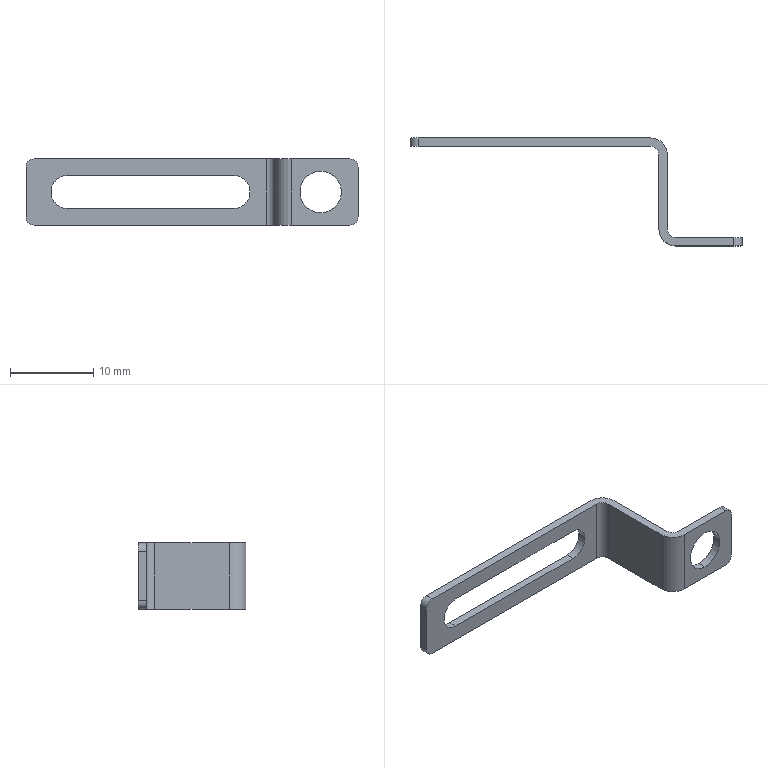Part | NX | features BREP 1 | 1 solid | 24 faces | box 40 x 13 x 8 mm | volume 292.639 mm3 | cylinder 12 | plane 12 | commonest cylinder face diameters 2 x6 4 x4 5 x2
STEP:
#1=CARTESIAN_POINT('',(5.5,0.,1.5));
#2=VERTEX_POINT('',#1);
#3=CARTESIAN_POINT('',(5.5,0.,6.5));
#4=VERTEX_POINT('',#3);
#5=CARTESIAN_POINT('',(5.5,0.,4.));
#6=DIRECTION('',(0.,1.,0.));
#7=DIRECTION('',(0.,0.,1.));
#8=AXIS2_PLACEMENT_3D('',#5,#6,#7);
#9=CIRCLE('',#8,2.5);
#10=EDGE_CURVE('',#2,#4,#9,.T.);
#11=ORIENTED_EDGE('',*,*,#10,.F.);
#12=CARTESIAN_POINT('',(5.5,1.,1.5));
#13=VERTEX_POINT('',#12);
#14=CARTESIAN_POINT('',(5.5,0.,1.5));
#15=DIRECTION('',(0.,1.,0.));
#16=VECTOR('',#15,1000.);
#17=LINE('',#14,#16);
#18=EDGE_CURVE('',#13,#2,#17,.F.);
#19=ORIENTED_EDGE('',*,*,#18,.F.);
#20=CARTESIAN_POINT('',(5.5,1.,6.5));
#21=VERTEX_POINT('',#20);
#22=CARTESIAN_POINT('',(5.5,1.,4.));
#23=DIRECTION('',(0.,1.,0.));
#24=DIRECTION('',(0.,0.,1.));
#25=AXIS2_PLACEMENT_3D('',#22,#23,#24);
#26=CIRCLE('',#25,2.5);
#27=EDGE_CURVE('',#13,#21,#26,.T.);
#28=ORIENTED_EDGE('',*,*,#27,.T.);
#29=CARTESIAN_POINT('',(5.5,0.,6.5));
#30=DIRECTION('',(0.,1.,0.));
#31=VECTOR('',#30,1000.);
#32=LINE('',#29,#31);
#33=EDGE_CURVE('',#21,#4,#32,.F.);
#34=ORIENTED_EDGE('',*,*,#33,.T.);
#35=EDGE_LOOP('',(#11,#19,#28,#34));
#36=FACE_BOUND('',#35,.T.);
#37=CARTESIAN_POINT('',(5.5,0.,4.));
#38=DIRECTION('',(0.,1.,0.));
#39=DIRECTION('',(0.,0.,1.));
#40=AXIS2_PLACEMENT_3D('',#37,#38,#39);
#41=CYLINDRICAL_SURFACE('',#40,2.5);
#42=ADVANCED_FACE('',(#36),#41,.F.);
#43=CARTESIAN_POINT('',(-1.,13.,8.));
#44=VERTEX_POINT('',#43);
#45=CARTESIAN_POINT('',(-29.,13.,8.));
#46=VERTEX_POINT('',#45);
#47=CARTESIAN_POINT('',(0.,13.,8.));
#48=DIRECTION('',(-1.,0.,0.));
#49=VECTOR('',#48,1000.);
#50=LINE('',#47,#49);
#51=EDGE_CURVE('',#44,#46,#50,.T.);
#52=ORIENTED_EDGE('',*,*,#51,.F.);
#53=CARTESIAN_POINT('',(-1.,13.,0.));
#54=VERTEX_POINT('',#53);
#55=CARTESIAN_POINT('',(-1.,13.,8.));
#56=DIRECTION('',(0.,0.,-1.));
#57=VECTOR('',#56,1000.);
#58=LINE('',#55,#57);
#59=EDGE_CURVE('',#44,#54,#58,.T.);
#60=ORIENTED_EDGE('',*,*,#59,.T.);
#61=CARTESIAN_POINT('',(-29.,13.,0.));
#62=VERTEX_POINT('',#61);
#63=CARTESIAN_POINT('',(0.,13.,0.));
#64=DIRECTION('',(-1.,0.,0.));
#65=VECTOR('',#64,1000.);
#66=LINE('',#63,#65);
#67=EDGE_CURVE('',#54,#62,#66,.T.);
#68=ORIENTED_EDGE('',*,*,#67,.T.);
#69=CARTESIAN_POINT('',(-30.,13.,1.));
#70=VERTEX_POINT('',#69);
#71=CARTESIAN_POINT('',(-29.,13.,1.));
#72=DIRECTION('',(0.,1.,0.));
#73=DIRECTION('',(1.,0.,0.));
#74=AXIS2_PLACEMENT_3D('',#71,#72,#73);
#75=CIRCLE('',#74,1.);
#76=EDGE_CURVE('',#62,#70,#75,.T.);
#77=ORIENTED_EDGE('',*,*,#76,.T.);
#78=CARTESIAN_POINT('',(-30.,13.,7.));
#79=VERTEX_POINT('',#78);
#80=CARTESIAN_POINT('',(-30.,13.,8.));
#81=DIRECTION('',(0.,0.,-1.));
#82=VECTOR('',#81,1000.);
#83=LINE('',#80,#82);
#84=EDGE_CURVE('',#79,#70,#83,.T.);
#85=ORIENTED_EDGE('',*,*,#84,.F.);
#86=CARTESIAN_POINT('',(-29.,13.,7.));
#87=DIRECTION('',(0.,1.,0.));
#88=DIRECTION('',(1.,0.,0.));
#89=AXIS2_PLACEMENT_3D('',#86,#87,#88);
#90=CIRCLE('',#89,1.);
#91=EDGE_CURVE('',#79,#46,#90,.T.);
#92=ORIENTED_EDGE('',*,*,#91,.T.);
#93=EDGE_LOOP('',(#52,#60,#68,#77,#85,#92));
#94=FACE_BOUND('',#93,.T.);
#95=CARTESIAN_POINT('',(-25.,13.,6.));
#96=VERTEX_POINT('',#95);
#97=CARTESIAN_POINT('',(-5.,13.,6.));
#98=VERTEX_POINT('',#97);
#99=CARTESIAN_POINT('',(-25.,13.,6.));
#100=DIRECTION('',(1.,0.,0.));
#101=VECTOR('',#100,1000.);
#102=LINE('',#99,#101);
#103=EDGE_CURVE('',#96,#98,#102,.T.);
#104=ORIENTED_EDGE('',*,*,#103,.F.);
#105=CARTESIAN_POINT('',(-25.,13.,2.));
#106=VERTEX_POINT('',#105);
#107=CARTESIAN_POINT('',(-25.,13.,4.));
#108=DIRECTION('',(0.,1.,0.));
#109=DIRECTION('',(0.,0.,1.));
#110=AXIS2_PLACEMENT_3D('',#107,#108,#109);
#111=CIRCLE('',#110,2.);
#112=EDGE_CURVE('',#106,#96,#111,.T.);
#113=ORIENTED_EDGE('',*,*,#112,.F.);
#114=CARTESIAN_POINT('',(-5.,13.,2.));
#115=VERTEX_POINT('',#114);
#116=CARTESIAN_POINT('',(-25.,13.,2.));
#117=DIRECTION('',(-1.,0.,0.));
#118=VECTOR('',#117,1000.);
#119=LINE('',#116,#118);
#120=EDGE_CURVE('',#115,#106,#119,.T.);
#121=ORIENTED_EDGE('',*,*,#120,.F.);
#122=CARTESIAN_POINT('',(-5.,13.,4.));
#123=DIRECTION('',(0.,1.,0.));
#124=DIRECTION('',(0.,0.,1.));
#125=AXIS2_PLACEMENT_3D('',#122,#123,#124);
#126=CIRCLE('',#125,2.);
#127=EDGE_CURVE('',#98,#115,#126,.T.);
#128=ORIENTED_EDGE('',*,*,#127,.F.);
#129=EDGE_LOOP('',(#104,#113,#121,#128));
#130=FACE_BOUND('',#129,.T.);
#131=CARTESIAN_POINT('',(0.,13.,8.));
#132=DIRECTION('',(0.,-1.,0.));
#133=DIRECTION('',(0.,0.,-1.));
#134=AXIS2_PLACEMENT_3D('',#131,#132,#133);
#135=PLANE('',#134);
#136=ADVANCED_FACE('',(#94,#130),#135,.F.);
#137=ORIENTED_EDGE('',*,*,#84,.T.);
#138=CARTESIAN_POINT('',(-30.,12.,1.));
#139=VERTEX_POINT('',#138);
#140=CARTESIAN_POINT('',(-30.,12.,1.));
#141=DIRECTION('',(0.,-1.,0.));
#142=VECTOR('',#141,1000.);
#143=LINE('',#140,#142);
#144=EDGE_CURVE('',#70,#139,#143,.T.);
#145=ORIENTED_EDGE('',*,*,#144,.T.);
#146=CARTESIAN_POINT('',(-30.,12.,7.));
#147=VERTEX_POINT('',#146);
#148=CARTESIAN_POINT('',(-30.,12.,8.));
#149=DIRECTION('',(0.,0.,-1.));
#150=VECTOR('',#149,1000.);
#151=LINE('',#148,#150);
#152=EDGE_CURVE('',#147,#139,#151,.T.);
#153=ORIENTED_EDGE('',*,*,#152,.F.);
#154=CARTESIAN_POINT('',(-30.,13.,7.));
#155=DIRECTION('',(0.,1.,0.));
#156=VECTOR('',#155,1000.);
#157=LINE('',#154,#156);
#158=EDGE_CURVE('',#147,#79,#157,.T.);
#159=ORIENTED_EDGE('',*,*,#158,.T.);
#160=EDGE_LOOP('',(#137,#145,#153,#159));
#161=FACE_BOUND('',#160,.T.);
#162=CARTESIAN_POINT('',(-30.,12.,8.));
#163=DIRECTION('',(-1.,0.,0.));
#164=DIRECTION('',(0.,0.,1.));
#165=AXIS2_PLACEMENT_3D('',#162,#163,#164);
#166=PLANE('',#165);
#167=ADVANCED_FACE('',(#161),#166,.T.);
#168=CARTESIAN_POINT('',(-1.,12.,0.));
#169=VERTEX_POINT('',#168);
#170=CARTESIAN_POINT('',(-29.,12.,0.));
#171=VERTEX_POINT('',#170);
#172=CARTESIAN_POINT('',(0.,12.,0.));
#173=DIRECTION('',(-1.,0.,0.));
#174=VECTOR('',#173,1000.);
#175=LINE('',#172,#174);
#176=EDGE_CURVE('',#169,#171,#175,.T.);
#177=ORIENTED_EDGE('',*,*,#176,.F.);
#178=CARTESIAN_POINT('',(-1.,12.,8.));
#179=VERTEX_POINT('',#178);
#180=CARTESIAN_POINT('',(-1.,12.,8.));
#181=DIRECTION('',(0.,0.,1.));
#182=VECTOR('',#181,1000.);
#183=LINE('',#180,#182);
#184=EDGE_CURVE('',#169,#179,#183,.T.);
#185=ORIENTED_EDGE('',*,*,#184,.T.);
#186=CARTESIAN_POINT('',(-29.,12.,8.));
#187=VERTEX_POINT('',#186);
#188=CARTESIAN_POINT('',(0.,12.,8.));
#189=DIRECTION('',(-1.,0.,0.));
#190=VECTOR('',#189,1000.);
#191=LINE('',#188,#190);
#192=EDGE_CURVE('',#179,#187,#191,.T.);
#193=ORIENTED_EDGE('',*,*,#192,.T.);
#194=CARTESIAN_POINT('',(-29.,12.,7.));
#195=DIRECTION('',(0.,-1.,0.));
#196=DIRECTION('',(1.,0.,0.));
#197=AXIS2_PLACEMENT_3D('',#194,#195,#196);
#198=CIRCLE('',#197,1.);
#199=EDGE_CURVE('',#187,#147,#198,.T.);
#200=ORIENTED_EDGE('',*,*,#199,.T.);
#201=ORIENTED_EDGE('',*,*,#152,.T.);
#202=CARTESIAN_POINT('',(-29.,12.,1.));
#203=DIRECTION('',(0.,-1.,0.));
#204=DIRECTION('',(1.,0.,0.));
#205=AXIS2_PLACEMENT_3D('',#202,#203,#204);
#206=CIRCLE('',#205,1.);
#207=EDGE_CURVE('',#139,#171,#206,.T.);
#208=ORIENTED_EDGE('',*,*,#207,.T.);
#209=EDGE_LOOP('',(#177,#185,#193,#200,#201,#208));
#210=FACE_BOUND('',#209,.T.);
#211=CARTESIAN_POINT('',(-25.,12.,6.));
#212=VERTEX_POINT('',#211);
#213=CARTESIAN_POINT('',(-25.,12.,2.));
#214=VERTEX_POINT('',#213);
#215=CARTESIAN_POINT('',(-25.,12.,4.));
#216=DIRECTION('',(0.,-1.,0.));
#217=DIRECTION('',(1.,0.,0.));
#218=AXIS2_PLACEMENT_3D('',#215,#216,#217);
#219=CIRCLE('',#218,2.);
#220=EDGE_CURVE('',#212,#214,#219,.T.);
#221=ORIENTED_EDGE('',*,*,#220,.F.);
#222=CARTESIAN_POINT('',(-5.,12.,6.));
#223=VERTEX_POINT('',#222);
#224=CARTESIAN_POINT('',(0.,12.,6.));
#225=DIRECTION('',(-1.,0.,0.));
#226=VECTOR('',#225,1000.);
#227=LINE('',#224,#226);
#228=EDGE_CURVE('',#223,#212,#227,.T.);
#229=ORIENTED_EDGE('',*,*,#228,.F.);
#230=CARTESIAN_POINT('',(-5.,12.,2.));
#231=VERTEX_POINT('',#230);
#232=CARTESIAN_POINT('',(-5.,12.,4.));
#233=DIRECTION('',(0.,-1.,0.));
#234=DIRECTION('',(1.,0.,0.));
#235=AXIS2_PLACEMENT_3D('',#232,#233,#234);
#236=CIRCLE('',#235,2.);
#237=EDGE_CURVE('',#231,#223,#236,.T.);
#238=ORIENTED_EDGE('',*,*,#237,.F.);
#239=CARTESIAN_POINT('',(0.,12.,2.));
#240=DIRECTION('',(1.,0.,0.));
#241=VECTOR('',#240,1000.);
#242=LINE('',#239,#241);
#243=EDGE_CURVE('',#214,#231,#242,.T.);
#244=ORIENTED_EDGE('',*,*,#243,.F.);
#245=EDGE_LOOP('',(#221,#229,#238,#244));
#246=FACE_BOUND('',#245,.T.);
#247=CARTESIAN_POINT('',(0.,12.,8.));
#248=DIRECTION('',(0.,-1.,0.));
#249=DIRECTION('',(0.,0.,-1.));
#250=AXIS2_PLACEMENT_3D('',#247,#248,#249);
#251=PLANE('',#250);
#252=ADVANCED_FACE('',(#210,#246),#251,.T.);
#253=CARTESIAN_POINT('',(0.,2.,0.));
#254=VERTEX_POINT('',#253);
#255=CARTESIAN_POINT('',(0.,11.,0.));
#256=VERTEX_POINT('',#255);
#257=CARTESIAN_POINT('',(0.,0.,0.));
#258=DIRECTION('',(0.,1.,0.));
#259=VECTOR('',#258,1000.);
#260=LINE('',#257,#259);
#261=EDGE_CURVE('',#254,#256,#260,.T.);
#262=ORIENTED_EDGE('',*,*,#261,.F.);
#263=CARTESIAN_POINT('',(0.,2.,8.));
#264=VERTEX_POINT('',#263);
#265=CARTESIAN_POINT('',(0.,2.,8.));
#266=DIRECTION('',(0.,0.,1.));
#267=VECTOR('',#266,1000.);
#268=LINE('',#265,#267);
#269=EDGE_CURVE('',#254,#264,#268,.T.);
#270=ORIENTED_EDGE('',*,*,#269,.T.);
#271=CARTESIAN_POINT('',(0.,11.,8.));
#272=VERTEX_POINT('',#271);
#273=CARTESIAN_POINT('',(0.,0.,8.));
#274=DIRECTION('',(0.,1.,0.));
#275=VECTOR('',#274,1000.);
#276=LINE('',#273,#275);
#277=EDGE_CURVE('',#264,#272,#276,.T.);
#278=ORIENTED_EDGE('',*,*,#277,.T.);
#279=CARTESIAN_POINT('',(0.,11.,0.));
#280=DIRECTION('',(0.,0.,-1.));
#281=VECTOR('',#280,1000.);
#282=LINE('',#279,#281);
#283=EDGE_CURVE('',#272,#256,#282,.T.);
#284=ORIENTED_EDGE('',*,*,#283,.T.);
#285=EDGE_LOOP('',(#262,#270,#278,#284));
#286=FACE_BOUND('',#285,.T.);
#287=CARTESIAN_POINT('',(0.,0.,8.));
#288=DIRECTION('',(-1.,0.,0.));
#289=DIRECTION('',(0.,0.,1.));
#290=AXIS2_PLACEMENT_3D('',#287,#288,#289);
#291=PLANE('',#290);
#292=ADVANCED_FACE('',(#286),#291,.T.);
#293=CARTESIAN_POINT('',(9.,0.,8.));
#294=VERTEX_POINT('',#293);
#295=CARTESIAN_POINT('',(2.,0.,8.));
#296=VERTEX_POINT('',#295);
#297=CARTESIAN_POINT('',(0.,0.,8.));
#298=DIRECTION('',(-1.,0.,0.));
#299=VECTOR('',#298,1000.);
#300=LINE('',#297,#299);
#301=EDGE_CURVE('',#294,#296,#300,.T.);
#302=ORIENTED_EDGE('',*,*,#301,.T.);
#303=CARTESIAN_POINT('',(2.,0.,0.));
#304=VERTEX_POINT('',#303);
#305=CARTESIAN_POINT('',(2.,0.,8.));
#306=DIRECTION('',(0.,0.,-1.));
#307=VECTOR('',#306,1000.);
#308=LINE('',#305,#307);
#309=EDGE_CURVE('',#296,#304,#308,.T.);
#310=ORIENTED_EDGE('',*,*,#309,.T.);
#311=CARTESIAN_POINT('',(9.,0.,0.));
#312=VERTEX_POINT('',#311);
#313=CARTESIAN_POINT('',(0.,0.,0.));
#314=DIRECTION('',(-1.,0.,0.));
#315=VECTOR('',#314,1000.);
#316=LINE('',#313,#315);
#317=EDGE_CURVE('',#312,#304,#316,.T.);
#318=ORIENTED_EDGE('',*,*,#317,.F.);
#319=CARTESIAN_POINT('',(10.,0.,1.));
#320=VERTEX_POINT('',#319);
#321=CARTESIAN_POINT('',(9.,0.,1.));
#322=DIRECTION('',(0.,-1.,0.));
#323=DIRECTION('',(0.,0.,-1.));
#324=AXIS2_PLACEMENT_3D('',#321,#322,#323);
#325=CIRCLE('',#324,1.);
#326=EDGE_CURVE('',#312,#320,#325,.T.);
#327=ORIENTED_EDGE('',*,*,#326,.T.);
#328=CARTESIAN_POINT('',(10.,0.,7.));
#329=VERTEX_POINT('',#328);
#330=CARTESIAN_POINT('',(10.,0.,8.));
#331=DIRECTION('',(0.,0.,-1.));
#332=VECTOR('',#331,1000.);
#333=LINE('',#330,#332);
#334=EDGE_CURVE('',#329,#320,#333,.T.);
#335=ORIENTED_EDGE('',*,*,#334,.F.);
#336=CARTESIAN_POINT('',(9.,0.,7.));
#337=DIRECTION('',(0.,-1.,0.));
#338=DIRECTION('',(0.,0.,-1.));
#339=AXIS2_PLACEMENT_3D('',#336,#337,#338);
#340=CIRCLE('',#339,1.);
#341=EDGE_CURVE('',#329,#294,#340,.T.);
#342=ORIENTED_EDGE('',*,*,#341,.T.);
#343=EDGE_LOOP('',(#302,#310,#318,#327,#335,#342));
#344=FACE_BOUND('',#343,.T.);
#345=CARTESIAN_POINT('',(5.5,0.,4.));
#346=DIRECTION('',(0.,1.,0.));
#347=DIRECTION('',(0.,0.,1.));
#348=AXIS2_PLACEMENT_3D('',#345,#346,#347);
#349=CIRCLE('',#348,2.5);
#350=EDGE_CURVE('',#4,#2,#349,.T.);
#351=ORIENTED_EDGE('',*,*,#350,.T.);
#352=ORIENTED_EDGE('',*,*,#10,.T.);
#353=EDGE_LOOP('',(#351,#352));
#354=FACE_BOUND('',#353,.T.);
#355=CARTESIAN_POINT('',(0.,0.,8.));
#356=DIRECTION('',(0.,-1.,0.));
#357=DIRECTION('',(0.,0.,-1.));
#358=AXIS2_PLACEMENT_3D('',#355,#356,#357);
#359=PLANE('',#358);
#360=ADVANCED_FACE('',(#344,#354),#359,.T.);
#361=CARTESIAN_POINT('',(10.,1.,7.));
#362=VERTEX_POINT('',#361);
#363=CARTESIAN_POINT('',(10.,1.,1.));
#364=VERTEX_POINT('',#363);
#365=CARTESIAN_POINT('',(10.,1.,8.));
#366=DIRECTION('',(0.,0.,-1.));
#367=VECTOR('',#366,1000.);
#368=LINE('',#365,#367);
#369=EDGE_CURVE('',#362,#364,#368,.T.);
#370=ORIENTED_EDGE('',*,*,#369,.F.);
#371=CARTESIAN_POINT('',(10.,0.,7.));
#372=DIRECTION('',(0.,-1.,0.));
#373=VECTOR('',#372,1000.);
#374=LINE('',#371,#373);
#375=EDGE_CURVE('',#362,#329,#374,.T.);
#376=ORIENTED_EDGE('',*,*,#375,.T.);
#377=ORIENTED_EDGE('',*,*,#334,.T.);
#378=CARTESIAN_POINT('',(10.,1.,1.));
#379=DIRECTION('',(0.,1.,0.));
#380=VECTOR('',#379,1000.);
#381=LINE('',#378,#380);
#382=EDGE_CURVE('',#320,#364,#381,.T.);
#383=ORIENTED_EDGE('',*,*,#382,.T.);
#384=EDGE_LOOP('',(#370,#376,#377,#383));
#385=FACE_BOUND('',#384,.T.);
#386=CARTESIAN_POINT('',(10.,1.,8.));
#387=DIRECTION('',(1.,0.,0.));
#388=DIRECTION('',(0.,1.,0.));
#389=AXIS2_PLACEMENT_3D('',#386,#387,#388);
#390=PLANE('',#389);
#391=ADVANCED_FACE('',(#385),#390,.T.);
#392=CARTESIAN_POINT('',(9.,1.,8.));
#393=VERTEX_POINT('',#392);
#394=CARTESIAN_POINT('',(2.,1.,8.));
#395=VERTEX_POINT('',#394);
#396=CARTESIAN_POINT('',(0.,1.,8.));
#397=DIRECTION('',(-1.,0.,0.));
#398=VECTOR('',#397,1000.);
#399=LINE('',#396,#398);
#400=EDGE_CURVE('',#393,#395,#399,.T.);
#401=ORIENTED_EDGE('',*,*,#400,.F.);
#402=CARTESIAN_POINT('',(9.,1.,7.));
#403=DIRECTION('',(0.,1.,0.));
#404=DIRECTION('',(0.,0.,-1.));
#405=AXIS2_PLACEMENT_3D('',#402,#403,#404);
#406=CIRCLE('',#405,1.);
#407=EDGE_CURVE('',#393,#362,#406,.T.);
#408=ORIENTED_EDGE('',*,*,#407,.T.);
#409=ORIENTED_EDGE('',*,*,#369,.T.);
#410=CARTESIAN_POINT('',(9.,1.,0.));
#411=VERTEX_POINT('',#410);
#412=CARTESIAN_POINT('',(9.,1.,1.));
#413=DIRECTION('',(0.,1.,0.));
#414=DIRECTION('',(0.,0.,-1.));
#415=AXIS2_PLACEMENT_3D('',#412,#413,#414);
#416=CIRCLE('',#415,1.);
#417=EDGE_CURVE('',#364,#411,#416,.T.);
#418=ORIENTED_EDGE('',*,*,#417,.T.);
#419=CARTESIAN_POINT('',(2.,1.,0.));
#420=VERTEX_POINT('',#419);
#421=CARTESIAN_POINT('',(0.,1.,0.));
#422=DIRECTION('',(-1.,0.,0.));
#423=VECTOR('',#422,1000.);
#424=LINE('',#421,#423);
#425=EDGE_CURVE('',#411,#420,#424,.T.);
#426=ORIENTED_EDGE('',*,*,#425,.T.);
#427=CARTESIAN_POINT('',(2.,1.,8.));
#428=DIRECTION('',(0.,0.,1.));
#429=VECTOR('',#428,1000.);
#430=LINE('',#427,#429);
#431=EDGE_CURVE('',#420,#395,#430,.T.);
#432=ORIENTED_EDGE('',*,*,#431,.T.);
#433=EDGE_LOOP('',(#401,#408,#409,#418,#426,#432));
#434=FACE_BOUND('',#433,.T.);
#435=CARTESIAN_POINT('',(5.5,1.,4.));
#436=DIRECTION('',(0.,1.,0.));
#437=DIRECTION('',(0.,0.,1.));
#438=AXIS2_PLACEMENT_3D('',#435,#436,#437);
#439=CIRCLE('',#438,2.5);
#440=EDGE_CURVE('',#21,#13,#439,.T.);
#441=ORIENTED_EDGE('',*,*,#440,.F.);
#442=ORIENTED_EDGE('',*,*,#27,.F.);
#443=EDGE_LOOP('',(#441,#442));
#444=FACE_BOUND('',#443,.T.);
#445=CARTESIAN_POINT('',(0.,1.,8.));
#446=DIRECTION('',(0.,-1.,0.));
#447=DIRECTION('',(0.,0.,-1.));
#448=AXIS2_PLACEMENT_3D('',#445,#446,#447);
#449=PLANE('',#448);
#450=ADVANCED_FACE('',(#434,#444),#449,.F.);
#451=CARTESIAN_POINT('',(1.,2.,0.));
#452=VERTEX_POINT('',#451);
#453=CARTESIAN_POINT('',(1.,11.,0.));
#454=VERTEX_POINT('',#453);
#455=CARTESIAN_POINT('',(1.,0.,0.));
#456=DIRECTION('',(0.,1.,0.));
#457=VECTOR('',#456,1000.);
#458=LINE('',#455,#457);
#459=EDGE_CURVE('',#452,#454,#458,.T.);
#460=ORIENTED_EDGE('',*,*,#459,.T.);
#461=CARTESIAN_POINT('',(1.,11.,8.));
#462=VERTEX_POINT('',#461);
#463=CARTESIAN_POINT('',(1.,11.,8.));
#464=DIRECTION('',(0.,0.,1.));
#465=VECTOR('',#464,1000.);
#466=LINE('',#463,#465);
#467=EDGE_CURVE('',#454,#462,#466,.T.);
#468=ORIENTED_EDGE('',*,*,#467,.T.);
#469=CARTESIAN_POINT('',(1.,2.,8.));
#470=VERTEX_POINT('',#469);
#471=CARTESIAN_POINT('',(1.,0.,8.));
#472=DIRECTION('',(0.,1.,0.));
#473=VECTOR('',#472,1000.);
#474=LINE('',#471,#473);
#475=EDGE_CURVE('',#470,#462,#474,.T.);
#476=ORIENTED_EDGE('',*,*,#475,.F.);
#477=CARTESIAN_POINT('',(1.,2.,0.));
#478=DIRECTION('',(0.,0.,-1.));
#479=VECTOR('',#478,1000.);
#480=LINE('',#477,#479);
#481=EDGE_CURVE('',#470,#452,#480,.T.);
#482=ORIENTED_EDGE('',*,*,#481,.T.);
#483=EDGE_LOOP('',(#460,#468,#476,#482));
#484=FACE_BOUND('',#483,.T.);
#485=CARTESIAN_POINT('',(1.,0.,8.));
#486=DIRECTION('',(-1.,0.,0.));
#487=DIRECTION('',(0.,0.,1.));
#488=AXIS2_PLACEMENT_3D('',#485,#486,#487);
#489=PLANE('',#488);
#490=ADVANCED_FACE('',(#484),#489,.F.);
#491=ORIENTED_EDGE('',*,*,#475,.T.);
#492=CARTESIAN_POINT('',(-1.,11.,8.));
#493=DIRECTION('',(0.,0.,1.));
#494=DIRECTION('',(-1.,0.,0.));
#495=AXIS2_PLACEMENT_3D('',#492,#493,#494);
#496=CIRCLE('',#495,2.);
#497=EDGE_CURVE('',#462,#44,#496,.T.);
#498=ORIENTED_EDGE('',*,*,#497,.T.);
#499=ORIENTED_EDGE('',*,*,#51,.T.);
#500=CARTESIAN_POINT('',(-29.,12.,8.));
#501=DIRECTION('',(0.,-1.,0.));
#502=VECTOR('',#501,1000.);
#503=LINE('',#500,#502);
#504=EDGE_CURVE('',#46,#187,#503,.T.);
#505=ORIENTED_EDGE('',*,*,#504,.T.);
#506=ORIENTED_EDGE('',*,*,#192,.F.);
#507=CARTESIAN_POINT('',(-1.,11.,8.));
#508=DIRECTION('',(0.,0.,-1.));
#509=DIRECTION('',(-1.,0.,0.));
#510=AXIS2_PLACEMENT_3D('',#507,#508,#509);
#511=CIRCLE('',#510,1.);
#512=EDGE_CURVE('',#179,#272,#511,.T.);
#513=ORIENTED_EDGE('',*,*,#512,.T.);
#514=ORIENTED_EDGE('',*,*,#277,.F.);
#515=CARTESIAN_POINT('',(2.,2.,8.));
#516=DIRECTION('',(0.,0.,1.));
#517=DIRECTION('',(-1.,0.,0.));
#518=AXIS2_PLACEMENT_3D('',#515,#516,#517);
#519=CIRCLE('',#518,2.);
#520=EDGE_CURVE('',#264,#296,#519,.T.);
#521=ORIENTED_EDGE('',*,*,#520,.T.);
#522=ORIENTED_EDGE('',*,*,#301,.F.);
#523=CARTESIAN_POINT('',(9.,1.,8.));
#524=DIRECTION('',(0.,1.,0.));
#525=VECTOR('',#524,1000.);
#526=LINE('',#523,#525);
#527=EDGE_CURVE('',#294,#393,#526,.T.);
#528=ORIENTED_EDGE('',*,*,#527,.T.);
#529=ORIENTED_EDGE('',*,*,#400,.T.);
#530=CARTESIAN_POINT('',(2.,2.,8.));
#531=DIRECTION('',(0.,0.,-1.));
#532=DIRECTION('',(-1.,0.,0.));
#533=AXIS2_PLACEMENT_3D('',#530,#531,#532);
#534=CIRCLE('',#533,1.);
#535=EDGE_CURVE('',#395,#470,#534,.T.);
#536=ORIENTED_EDGE('',*,*,#535,.T.);
#537=EDGE_LOOP('',(#491,#498,#499,#505,#506,#513,#514,#521,#522,#528,#529,#536));
#538=FACE_BOUND('',#537,.T.);
#539=CARTESIAN_POINT('',(0.,0.,8.));
#540=DIRECTION('',(0.,0.,-1.));
#541=DIRECTION('',(0.,-1.,0.));
#542=AXIS2_PLACEMENT_3D('',#539,#540,#541);
#543=PLANE('',#542);
#544=ADVANCED_FACE('',(#538),#543,.F.);
#545=ORIENTED_EDGE('',*,*,#67,.F.);
#546=CARTESIAN_POINT('',(-1.,11.,0.));
#547=DIRECTION('',(0.,0.,-1.));
#548=DIRECTION('',(-1.,0.,0.));
#549=AXIS2_PLACEMENT_3D('',#546,#547,#548);
#550=CIRCLE('',#549,2.);
#551=EDGE_CURVE('',#54,#454,#550,.T.);
#552=ORIENTED_EDGE('',*,*,#551,.T.);
#553=ORIENTED_EDGE('',*,*,#459,.F.);
#554=CARTESIAN_POINT('',(2.,2.,0.));
#555=DIRECTION('',(0.,0.,1.));
#556=DIRECTION('',(-1.,0.,0.));
#557=AXIS2_PLACEMENT_3D('',#554,#555,#556);
#558=CIRCLE('',#557,1.);
#559=EDGE_CURVE('',#452,#420,#558,.T.);
#560=ORIENTED_EDGE('',*,*,#559,.T.);
#561=ORIENTED_EDGE('',*,*,#425,.F.);
#562=CARTESIAN_POINT('',(9.,0.,0.));
#563=DIRECTION('',(0.,-1.,0.));
#564=VECTOR('',#563,1000.);
#565=LINE('',#562,#564);
#566=EDGE_CURVE('',#411,#312,#565,.T.);
#567=ORIENTED_EDGE('',*,*,#566,.T.);
#568=ORIENTED_EDGE('',*,*,#317,.T.);
#569=CARTESIAN_POINT('',(2.,2.,0.));
#570=DIRECTION('',(0.,0.,-1.));
#571=DIRECTION('',(-1.,0.,0.));
#572=AXIS2_PLACEMENT_3D('',#569,#570,#571);
#573=CIRCLE('',#572,2.);
#574=EDGE_CURVE('',#304,#254,#573,.T.);
#575=ORIENTED_EDGE('',*,*,#574,.T.);
#576=ORIENTED_EDGE('',*,*,#261,.T.);
#577=CARTESIAN_POINT('',(-1.,11.,0.));
#578=DIRECTION('',(0.,0.,1.));
#579=DIRECTION('',(-1.,0.,0.));
#580=AXIS2_PLACEMENT_3D('',#577,#578,#579);
#581=CIRCLE('',#580,1.);
#582=EDGE_CURVE('',#256,#169,#581,.T.);
#583=ORIENTED_EDGE('',*,*,#582,.T.);
#584=ORIENTED_EDGE('',*,*,#176,.T.);
#585=CARTESIAN_POINT('',(-29.,0.,0.));
#586=DIRECTION('',(0.,1.,0.));
#587=VECTOR('',#586,1000.);
#588=LINE('',#585,#587);
#589=EDGE_CURVE('',#171,#62,#588,.T.);
#590=ORIENTED_EDGE('',*,*,#589,.T.);
#591=EDGE_LOOP('',(#545,#552,#553,#560,#561,#567,#568,#575,#576,#583,#584,#590));
#592=FACE_BOUND('',#591,.T.);
#593=CARTESIAN_POINT('',(0.,0.,0.));
#594=DIRECTION('',(0.,0.,-1.));
#595=DIRECTION('',(0.,-1.,0.));
#596=AXIS2_PLACEMENT_3D('',#593,#594,#595);
#597=PLANE('',#596);
#598=ADVANCED_FACE('',(#592),#597,.T.);
#599=ORIENTED_EDGE('',*,*,#220,.T.);
#600=CARTESIAN_POINT('',(-25.,5.,2.));
#601=DIRECTION('',(0.,1.,0.));
#602=VECTOR('',#601,1000.);
#603=LINE('',#600,#602);
#604=EDGE_CURVE('',#214,#106,#603,.T.);
#605=ORIENTED_EDGE('',*,*,#604,.T.);
#606=ORIENTED_EDGE('',*,*,#112,.T.);
#607=CARTESIAN_POINT('',(-25.,5.,6.));
#608=DIRECTION('',(0.,1.,0.));
#609=VECTOR('',#608,1000.);
#610=LINE('',#607,#609);
#611=EDGE_CURVE('',#212,#96,#610,.T.);
#612=ORIENTED_EDGE('',*,*,#611,.F.);
#613=EDGE_LOOP('',(#599,#605,#606,#612));
#614=FACE_BOUND('',#613,.T.);
#615=CARTESIAN_POINT('',(-25.,5.,4.));
#616=DIRECTION('',(0.,1.,0.));
#617=DIRECTION('',(0.,0.,1.));
#618=AXIS2_PLACEMENT_3D('',#615,#616,#617);
#619=CYLINDRICAL_SURFACE('',#618,2.);
#620=ADVANCED_FACE('',(#614),#619,.F.);
#621=ORIENTED_EDGE('',*,*,#243,.T.);
#622=CARTESIAN_POINT('',(-5.,5.,2.));
#623=DIRECTION('',(0.,1.,0.));
#624=VECTOR('',#623,1000.);
#625=LINE('',#622,#624);
#626=EDGE_CURVE('',#231,#115,#625,.T.);
#627=ORIENTED_EDGE('',*,*,#626,.T.);
#628=ORIENTED_EDGE('',*,*,#120,.T.);
#629=ORIENTED_EDGE('',*,*,#604,.F.);
#630=EDGE_LOOP('',(#621,#627,#628,#629));
#631=FACE_BOUND('',#630,.T.);
#632=CARTESIAN_POINT('',(-25.,5.,2.));
#633=DIRECTION('',(0.,0.,-1.));
#634=DIRECTION('',(-1.,0.,0.));
#635=AXIS2_PLACEMENT_3D('',#632,#633,#634);
#636=PLANE('',#635);
#637=ADVANCED_FACE('',(#631),#636,.F.);
#638=ORIENTED_EDGE('',*,*,#237,.T.);
#639=CARTESIAN_POINT('',(-5.,5.,6.));
#640=DIRECTION('',(0.,1.,0.));
#641=VECTOR('',#640,1000.);
#642=LINE('',#639,#641);
#643=EDGE_CURVE('',#223,#98,#642,.T.);
#644=ORIENTED_EDGE('',*,*,#643,.T.);
#645=ORIENTED_EDGE('',*,*,#127,.T.);
#646=ORIENTED_EDGE('',*,*,#626,.F.);
#647=EDGE_LOOP('',(#638,#644,#645,#646));
#648=FACE_BOUND('',#647,.T.);
#649=CARTESIAN_POINT('',(-5.,5.,4.));
#650=DIRECTION('',(0.,1.,0.));
#651=DIRECTION('',(0.,0.,1.));
#652=AXIS2_PLACEMENT_3D('',#649,#650,#651);
#653=CYLINDRICAL_SURFACE('',#652,2.);
#654=ADVANCED_FACE('',(#648),#653,.F.);
#655=ORIENTED_EDGE('',*,*,#228,.T.);
#656=ORIENTED_EDGE('',*,*,#611,.T.);
#657=ORIENTED_EDGE('',*,*,#103,.T.);
#658=ORIENTED_EDGE('',*,*,#643,.F.);
#659=EDGE_LOOP('',(#655,#656,#657,#658));
#660=FACE_BOUND('',#659,.T.);
#661=CARTESIAN_POINT('',(-25.,5.,6.));
#662=DIRECTION('',(0.,0.,1.));
#663=DIRECTION('',(1.,0.,0.));
#664=AXIS2_PLACEMENT_3D('',#661,#662,#663);
#665=PLANE('',#664);
#666=ADVANCED_FACE('',(#660),#665,.F.);
#667=ORIENTED_EDGE('',*,*,#18,.T.);
#668=ORIENTED_EDGE('',*,*,#350,.F.);
#669=ORIENTED_EDGE('',*,*,#33,.F.);
#670=ORIENTED_EDGE('',*,*,#440,.T.);
#671=EDGE_LOOP('',(#667,#668,#669,#670));
#672=FACE_BOUND('',#671,.T.);
#673=CARTESIAN_POINT('',(5.5,0.,4.));
#674=DIRECTION('',(0.,1.,0.));
#675=DIRECTION('',(0.,0.,1.));
#676=AXIS2_PLACEMENT_3D('',#673,#674,#675);
#677=CYLINDRICAL_SURFACE('',#676,2.5);
#678=ADVANCED_FACE('',(#672),#677,.F.);
#679=ORIENTED_EDGE('',*,*,#407,.F.);
#680=ORIENTED_EDGE('',*,*,#527,.F.);
#681=ORIENTED_EDGE('',*,*,#341,.F.);
#682=ORIENTED_EDGE('',*,*,#375,.F.);
#683=EDGE_LOOP('',(#679,#680,#681,#682));
#684=FACE_BOUND('',#683,.T.);
#685=CARTESIAN_POINT('',(9.,1.,7.));
#686=DIRECTION('',(0.,1.,0.));
#687=DIRECTION('',(0.,0.,1.));
#688=AXIS2_PLACEMENT_3D('',#685,#686,#687);
#689=CYLINDRICAL_SURFACE('',#688,1.);
#690=ADVANCED_FACE('',(#684),#689,.T.);
#691=ORIENTED_EDGE('',*,*,#417,.F.);
#692=ORIENTED_EDGE('',*,*,#382,.F.);
#693=ORIENTED_EDGE('',*,*,#326,.F.);
#694=ORIENTED_EDGE('',*,*,#566,.F.);
#695=EDGE_LOOP('',(#691,#692,#693,#694));
#696=FACE_BOUND('',#695,.T.);
#697=CARTESIAN_POINT('',(9.,0.,1.));
#698=DIRECTION('',(0.,-1.,0.));
#699=DIRECTION('',(0.,0.,-1.));
#700=AXIS2_PLACEMENT_3D('',#697,#698,#699);
#701=CYLINDRICAL_SURFACE('',#700,1.);
#702=ADVANCED_FACE('',(#696),#701,.T.);
#703=ORIENTED_EDGE('',*,*,#535,.F.);
#704=ORIENTED_EDGE('',*,*,#431,.F.);
#705=ORIENTED_EDGE('',*,*,#559,.F.);
#706=ORIENTED_EDGE('',*,*,#481,.F.);
#707=EDGE_LOOP('',(#703,#704,#705,#706));
#708=FACE_BOUND('',#707,.T.);
#709=CARTESIAN_POINT('',(2.,2.,8.));
#710=DIRECTION('',(0.,0.,1.));
#711=DIRECTION('',(1.,0.,0.));
#712=AXIS2_PLACEMENT_3D('',#709,#710,#711);
#713=CYLINDRICAL_SURFACE('',#712,1.);
#714=ADVANCED_FACE('',(#708),#713,.F.);
#715=ORIENTED_EDGE('',*,*,#512,.F.);
#716=ORIENTED_EDGE('',*,*,#184,.F.);
#717=ORIENTED_EDGE('',*,*,#582,.F.);
#718=ORIENTED_EDGE('',*,*,#283,.F.);
#719=EDGE_LOOP('',(#715,#716,#717,#718));
#720=FACE_BOUND('',#719,.T.);
#721=CARTESIAN_POINT('',(-1.,11.,8.));
#722=DIRECTION('',(0.,0.,1.));
#723=DIRECTION('',(1.,0.,0.));
#724=AXIS2_PLACEMENT_3D('',#721,#722,#723);
#725=CYLINDRICAL_SURFACE('',#724,1.);
#726=ADVANCED_FACE('',(#720),#725,.F.);
#727=ORIENTED_EDGE('',*,*,#207,.F.);
#728=ORIENTED_EDGE('',*,*,#144,.F.);
#729=ORIENTED_EDGE('',*,*,#76,.F.);
#730=ORIENTED_EDGE('',*,*,#589,.F.);
#731=EDGE_LOOP('',(#727,#728,#729,#730));
#732=FACE_BOUND('',#731,.T.);
#733=CARTESIAN_POINT('',(-29.,0.,1.));
#734=DIRECTION('',(0.,1.,0.));
#735=DIRECTION('',(0.,0.,1.));
#736=AXIS2_PLACEMENT_3D('',#733,#734,#735);
#737=CYLINDRICAL_SURFACE('',#736,1.);
#738=ADVANCED_FACE('',(#732),#737,.T.);
#739=ORIENTED_EDGE('',*,*,#199,.F.);
#740=ORIENTED_EDGE('',*,*,#504,.F.);
#741=ORIENTED_EDGE('',*,*,#91,.F.);
#742=ORIENTED_EDGE('',*,*,#158,.F.);
#743=EDGE_LOOP('',(#739,#740,#741,#742));
#744=FACE_BOUND('',#743,.T.);
#745=CARTESIAN_POINT('',(-29.,12.,7.));
#746=DIRECTION('',(0.,-1.,0.));
#747=DIRECTION('',(0.,0.,-1.));
#748=AXIS2_PLACEMENT_3D('',#745,#746,#747);
#749=CYLINDRICAL_SURFACE('',#748,1.);
#750=ADVANCED_FACE('',(#744),#749,.T.);
#751=ORIENTED_EDGE('',*,*,#497,.F.);
#752=ORIENTED_EDGE('',*,*,#467,.F.);
#753=ORIENTED_EDGE('',*,*,#551,.F.);
#754=ORIENTED_EDGE('',*,*,#59,.F.);
#755=EDGE_LOOP('',(#751,#752,#753,#754));
#756=FACE_BOUND('',#755,.T.);
#757=CARTESIAN_POINT('',(-1.,11.,8.));
#758=DIRECTION('',(0.,0.,-1.));
#759=DIRECTION('',(-1.,0.,0.));
#760=AXIS2_PLACEMENT_3D('',#757,#758,#759);
#761=CYLINDRICAL_SURFACE('',#760,2.);
#762=ADVANCED_FACE('',(#756),#761,.T.);
#763=ORIENTED_EDGE('',*,*,#520,.F.);
#764=ORIENTED_EDGE('',*,*,#269,.F.);
#765=ORIENTED_EDGE('',*,*,#574,.F.);
#766=ORIENTED_EDGE('',*,*,#309,.F.);
#767=EDGE_LOOP('',(#763,#764,#765,#766));
#768=FACE_BOUND('',#767,.T.);
#769=CARTESIAN_POINT('',(2.,2.,8.));
#770=DIRECTION('',(0.,0.,-1.));
#771=DIRECTION('',(-1.,0.,0.));
#772=AXIS2_PLACEMENT_3D('',#769,#770,#771);
#773=CYLINDRICAL_SURFACE('',#772,2.);
#774=ADVANCED_FACE('',(#768),#773,.T.);
#775=CLOSED_SHELL('',(#42,#136,#167,#252,#292,#360,#391,#450,#490,#544,#598,#620,#637,#654,#666,#678,#690,#702,#714,#726,#738,#750,#762,#774));
#776=MANIFOLD_SOLID_BREP('',#775);
#777=(LENGTH_UNIT()NAMED_UNIT(*)SI_UNIT(.MILLI.,.METRE.));
#778=UNCERTAINTY_MEASURE_WITH_UNIT(LENGTH_MEASURE(0.00001),#777,'','');
#779=(NAMED_UNIT(*)PLANE_ANGLE_UNIT()SI_UNIT($,.RADIAN.));
#780=(NAMED_UNIT(*)SI_UNIT($,.STERADIAN.)SOLID_ANGLE_UNIT());
#781=(GEOMETRIC_REPRESENTATION_CONTEXT(3)GLOBAL_UNCERTAINTY_ASSIGNED_CONTEXT((#778))GLOBAL_UNIT_ASSIGNED_CONTEXT((#777,#779,#780))REPRESENTATION_CONTEXT('',''));
#782=ADVANCED_BREP_SHAPE_REPRESENTATION('',(#776),#781);